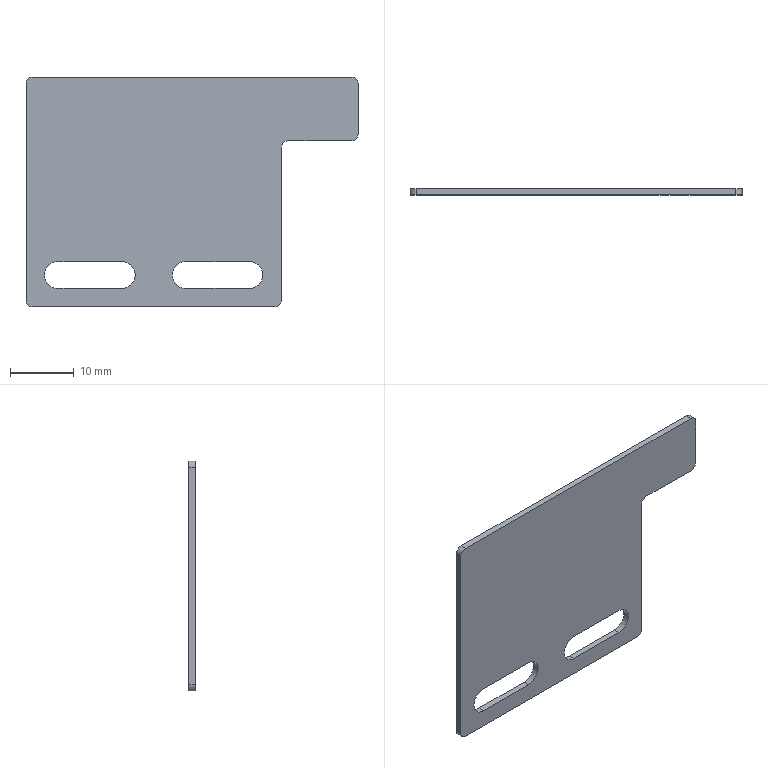Part | NX | features BREP 1 | 1 solid | 24 faces | box 52 x 1 x 36 mm | volume 1447 mm3 | cylinder 12 | plane 12 | commonest cylinder face diameters 2 x6 4.2 x6
STEP:
#1=CARTESIAN_POINT('',(20.,0.,1.));
#2=VERTEX_POINT('',#1);
#3=CARTESIAN_POINT('',(19.,0.,0.));
#4=VERTEX_POINT('',#3);
#5=CARTESIAN_POINT('',(19.,0.,1.));
#6=DIRECTION('',(0.,1.,0.));
#7=DIRECTION('',(-1.,0.,0.));
#8=AXIS2_PLACEMENT_3D('',#5,#6,#7);
#9=CIRCLE('',#8,1.);
#10=EDGE_CURVE('',#2,#4,#9,.T.);
#11=ORIENTED_EDGE('',*,*,#10,.F.);
#12=CARTESIAN_POINT('',(20.,-1.,1.));
#13=VERTEX_POINT('',#12);
#14=CARTESIAN_POINT('',(20.,0.,1.));
#15=DIRECTION('',(0.,1.,0.));
#16=VECTOR('',#15,1000.);
#17=LINE('',#14,#16);
#18=EDGE_CURVE('',#13,#2,#17,.T.);
#19=ORIENTED_EDGE('',*,*,#18,.F.);
#20=CARTESIAN_POINT('',(19.,-1.,0.));
#21=VERTEX_POINT('',#20);
#22=CARTESIAN_POINT('',(19.,-1.,1.));
#23=DIRECTION('',(0.,-1.,0.));
#24=DIRECTION('',(-1.,0.,0.));
#25=AXIS2_PLACEMENT_3D('',#22,#23,#24);
#26=CIRCLE('',#25,1.);
#27=EDGE_CURVE('',#21,#13,#26,.T.);
#28=ORIENTED_EDGE('',*,*,#27,.F.);
#29=CARTESIAN_POINT('',(19.,0.,0.));
#30=DIRECTION('',(0.,-1.,0.));
#31=VECTOR('',#30,1000.);
#32=LINE('',#29,#31);
#33=EDGE_CURVE('',#4,#21,#32,.T.);
#34=ORIENTED_EDGE('',*,*,#33,.F.);
#35=EDGE_LOOP('',(#11,#19,#28,#34));
#36=FACE_BOUND('',#35,.T.);
#37=CARTESIAN_POINT('',(19.,0.,1.));
#38=DIRECTION('',(0.,-1.,0.));
#39=DIRECTION('',(0.,0.,-1.));
#40=AXIS2_PLACEMENT_3D('',#37,#38,#39);
#41=CYLINDRICAL_SURFACE('',#40,1.);
#42=ADVANCED_FACE('',(#36),#41,.T.);
#43=CARTESIAN_POINT('',(-20.,-1.,1.));
#44=VERTEX_POINT('',#43);
#45=CARTESIAN_POINT('',(-19.,-1.,0.));
#46=VERTEX_POINT('',#45);
#47=CARTESIAN_POINT('',(-19.,-1.,1.));
#48=DIRECTION('',(0.,-1.,0.));
#49=DIRECTION('',(-1.,0.,0.));
#50=AXIS2_PLACEMENT_3D('',#47,#48,#49);
#51=CIRCLE('',#50,1.);
#52=EDGE_CURVE('',#44,#46,#51,.T.);
#53=ORIENTED_EDGE('',*,*,#52,.F.);
#54=CARTESIAN_POINT('',(-20.,0.,1.));
#55=VERTEX_POINT('',#54);
#56=CARTESIAN_POINT('',(-20.,-1.,1.));
#57=DIRECTION('',(0.,-1.,0.));
#58=VECTOR('',#57,1000.);
#59=LINE('',#56,#58);
#60=EDGE_CURVE('',#55,#44,#59,.T.);
#61=ORIENTED_EDGE('',*,*,#60,.F.);
#62=CARTESIAN_POINT('',(-19.,0.,0.));
#63=VERTEX_POINT('',#62);
#64=CARTESIAN_POINT('',(-19.,0.,1.));
#65=DIRECTION('',(0.,1.,0.));
#66=DIRECTION('',(-1.,0.,0.));
#67=AXIS2_PLACEMENT_3D('',#64,#65,#66);
#68=CIRCLE('',#67,1.);
#69=EDGE_CURVE('',#63,#55,#68,.T.);
#70=ORIENTED_EDGE('',*,*,#69,.F.);
#71=CARTESIAN_POINT('',(-19.,0.,0.));
#72=DIRECTION('',(0.,1.,0.));
#73=VECTOR('',#72,1000.);
#74=LINE('',#71,#73);
#75=EDGE_CURVE('',#46,#63,#74,.T.);
#76=ORIENTED_EDGE('',*,*,#75,.F.);
#77=EDGE_LOOP('',(#53,#61,#70,#76));
#78=FACE_BOUND('',#77,.T.);
#79=CARTESIAN_POINT('',(-19.,0.,1.));
#80=DIRECTION('',(0.,1.,0.));
#81=DIRECTION('',(0.,0.,1.));
#82=AXIS2_PLACEMENT_3D('',#79,#80,#81);
#83=CYLINDRICAL_SURFACE('',#82,1.);
#84=ADVANCED_FACE('',(#78),#83,.T.);
#85=CARTESIAN_POINT('',(20.,-1.,25.));
#86=VERTEX_POINT('',#85);
#87=CARTESIAN_POINT('',(21.,-1.,26.));
#88=VERTEX_POINT('',#87);
#89=CARTESIAN_POINT('',(21.,-1.,25.));
#90=DIRECTION('',(0.,1.,0.));
#91=DIRECTION('',(-1.,0.,0.));
#92=AXIS2_PLACEMENT_3D('',#89,#90,#91);
#93=CIRCLE('',#92,1.);
#94=EDGE_CURVE('',#86,#88,#93,.T.);
#95=ORIENTED_EDGE('',*,*,#94,.F.);
#96=CARTESIAN_POINT('',(20.,0.,25.));
#97=VERTEX_POINT('',#96);
#98=CARTESIAN_POINT('',(20.,-1.,25.));
#99=DIRECTION('',(0.,-1.,0.));
#100=VECTOR('',#99,1000.);
#101=LINE('',#98,#100);
#102=EDGE_CURVE('',#97,#86,#101,.T.);
#103=ORIENTED_EDGE('',*,*,#102,.F.);
#104=CARTESIAN_POINT('',(21.,0.,26.));
#105=VERTEX_POINT('',#104);
#106=CARTESIAN_POINT('',(21.,0.,25.));
#107=DIRECTION('',(0.,-1.,0.));
#108=DIRECTION('',(-1.,0.,0.));
#109=AXIS2_PLACEMENT_3D('',#106,#107,#108);
#110=CIRCLE('',#109,1.);
#111=EDGE_CURVE('',#105,#97,#110,.T.);
#112=ORIENTED_EDGE('',*,*,#111,.F.);
#113=CARTESIAN_POINT('',(21.,0.,26.));
#114=DIRECTION('',(0.,1.,0.));
#115=VECTOR('',#114,1000.);
#116=LINE('',#113,#115);
#117=EDGE_CURVE('',#88,#105,#116,.T.);
#118=ORIENTED_EDGE('',*,*,#117,.F.);
#119=EDGE_LOOP('',(#95,#103,#112,#118));
#120=FACE_BOUND('',#119,.T.);
#121=CARTESIAN_POINT('',(21.,-1.,25.));
#122=DIRECTION('',(0.,-1.,0.));
#123=DIRECTION('',(0.,0.,-1.));
#124=AXIS2_PLACEMENT_3D('',#121,#122,#123);
#125=CYLINDRICAL_SURFACE('',#124,1.);
#126=ADVANCED_FACE('',(#120),#125,.F.);
#127=CARTESIAN_POINT('',(31.,-1.,26.));
#128=VERTEX_POINT('',#127);
#129=CARTESIAN_POINT('',(32.,-1.,27.));
#130=VERTEX_POINT('',#129);
#131=CARTESIAN_POINT('',(31.,-1.,27.));
#132=DIRECTION('',(0.,-1.,0.));
#133=DIRECTION('',(-1.,0.,0.));
#134=AXIS2_PLACEMENT_3D('',#131,#132,#133);
#135=CIRCLE('',#134,1.);
#136=EDGE_CURVE('',#128,#130,#135,.T.);
#137=ORIENTED_EDGE('',*,*,#136,.F.);
#138=CARTESIAN_POINT('',(31.,0.,26.));
#139=VERTEX_POINT('',#138);
#140=CARTESIAN_POINT('',(31.,-1.,26.));
#141=DIRECTION('',(0.,-1.,0.));
#142=VECTOR('',#141,1000.);
#143=LINE('',#140,#142);
#144=EDGE_CURVE('',#139,#128,#143,.T.);
#145=ORIENTED_EDGE('',*,*,#144,.F.);
#146=CARTESIAN_POINT('',(32.,0.,27.));
#147=VERTEX_POINT('',#146);
#148=CARTESIAN_POINT('',(31.,0.,27.));
#149=DIRECTION('',(0.,1.,0.));
#150=DIRECTION('',(-1.,0.,0.));
#151=AXIS2_PLACEMENT_3D('',#148,#149,#150);
#152=CIRCLE('',#151,1.);
#153=EDGE_CURVE('',#147,#139,#152,.T.);
#154=ORIENTED_EDGE('',*,*,#153,.F.);
#155=CARTESIAN_POINT('',(32.,-1.,27.));
#156=DIRECTION('',(0.,1.,0.));
#157=VECTOR('',#156,1000.);
#158=LINE('',#155,#157);
#159=EDGE_CURVE('',#130,#147,#158,.T.);
#160=ORIENTED_EDGE('',*,*,#159,.F.);
#161=EDGE_LOOP('',(#137,#145,#154,#160));
#162=FACE_BOUND('',#161,.T.);
#163=CARTESIAN_POINT('',(31.,-1.,27.));
#164=DIRECTION('',(0.,1.,0.));
#165=DIRECTION('',(-1.,0.,0.));
#166=AXIS2_PLACEMENT_3D('',#163,#164,#165);
#167=CYLINDRICAL_SURFACE('',#166,1.);
#168=ADVANCED_FACE('',(#162),#167,.T.);
#169=CARTESIAN_POINT('',(32.,-1.,35.));
#170=VERTEX_POINT('',#169);
#171=CARTESIAN_POINT('',(31.,-1.,36.));
#172=VERTEX_POINT('',#171);
#173=CARTESIAN_POINT('',(31.,-1.,35.));
#174=DIRECTION('',(0.,-1.,0.));
#175=DIRECTION('',(-1.,0.,0.));
#176=AXIS2_PLACEMENT_3D('',#173,#174,#175);
#177=CIRCLE('',#176,1.);
#178=EDGE_CURVE('',#170,#172,#177,.T.);
#179=ORIENTED_EDGE('',*,*,#178,.F.);
#180=CARTESIAN_POINT('',(32.,0.,35.));
#181=VERTEX_POINT('',#180);
#182=CARTESIAN_POINT('',(32.,-1.,35.));
#183=DIRECTION('',(0.,-1.,0.));
#184=VECTOR('',#183,1000.);
#185=LINE('',#182,#184);
#186=EDGE_CURVE('',#181,#170,#185,.T.);
#187=ORIENTED_EDGE('',*,*,#186,.F.);
#188=CARTESIAN_POINT('',(31.,0.,36.));
#189=VERTEX_POINT('',#188);
#190=CARTESIAN_POINT('',(31.,0.,35.));
#191=DIRECTION('',(0.,1.,0.));
#192=DIRECTION('',(-1.,0.,0.));
#193=AXIS2_PLACEMENT_3D('',#190,#191,#192);
#194=CIRCLE('',#193,1.);
#195=EDGE_CURVE('',#189,#181,#194,.T.);
#196=ORIENTED_EDGE('',*,*,#195,.F.);
#197=CARTESIAN_POINT('',(31.,0.,36.));
#198=DIRECTION('',(0.,1.,0.));
#199=VECTOR('',#198,1000.);
#200=LINE('',#197,#199);
#201=EDGE_CURVE('',#172,#189,#200,.T.);
#202=ORIENTED_EDGE('',*,*,#201,.F.);
#203=EDGE_LOOP('',(#179,#187,#196,#202));
#204=FACE_BOUND('',#203,.T.);
#205=CARTESIAN_POINT('',(31.,0.,35.));
#206=DIRECTION('',(0.,-1.,0.));
#207=DIRECTION('',(1.,0.,0.));
#208=AXIS2_PLACEMENT_3D('',#205,#206,#207);
#209=CYLINDRICAL_SURFACE('',#208,1.);
#210=ADVANCED_FACE('',(#204),#209,.T.);
#211=CARTESIAN_POINT('',(-19.,-1.,36.));
#212=VERTEX_POINT('',#211);
#213=CARTESIAN_POINT('',(-20.,-1.,35.));
#214=VERTEX_POINT('',#213);
#215=CARTESIAN_POINT('',(-19.,-1.,35.));
#216=DIRECTION('',(0.,-1.,0.));
#217=DIRECTION('',(-1.,0.,0.));
#218=AXIS2_PLACEMENT_3D('',#215,#216,#217);
#219=CIRCLE('',#218,1.);
#220=EDGE_CURVE('',#212,#214,#219,.T.);
#221=ORIENTED_EDGE('',*,*,#220,.F.);
#222=CARTESIAN_POINT('',(-19.,0.,36.));
#223=VERTEX_POINT('',#222);
#224=CARTESIAN_POINT('',(-19.,-1.,36.));
#225=DIRECTION('',(0.,-1.,0.));
#226=VECTOR('',#225,1000.);
#227=LINE('',#224,#226);
#228=EDGE_CURVE('',#223,#212,#227,.T.);
#229=ORIENTED_EDGE('',*,*,#228,.F.);
#230=CARTESIAN_POINT('',(-20.,0.,35.));
#231=VERTEX_POINT('',#230);
#232=CARTESIAN_POINT('',(-19.,0.,35.));
#233=DIRECTION('',(0.,1.,0.));
#234=DIRECTION('',(-1.,0.,0.));
#235=AXIS2_PLACEMENT_3D('',#232,#233,#234);
#236=CIRCLE('',#235,1.);
#237=EDGE_CURVE('',#231,#223,#236,.T.);
#238=ORIENTED_EDGE('',*,*,#237,.F.);
#239=CARTESIAN_POINT('',(-20.,0.,35.));
#240=DIRECTION('',(0.,1.,0.));
#241=VECTOR('',#240,1000.);
#242=LINE('',#239,#241);
#243=EDGE_CURVE('',#214,#231,#242,.T.);
#244=ORIENTED_EDGE('',*,*,#243,.F.);
#245=EDGE_LOOP('',(#221,#229,#238,#244));
#246=FACE_BOUND('',#245,.T.);
#247=CARTESIAN_POINT('',(-19.,-1.,35.));
#248=DIRECTION('',(0.,-1.,0.));
#249=DIRECTION('',(0.,0.,-1.));
#250=AXIS2_PLACEMENT_3D('',#247,#248,#249);
#251=CYLINDRICAL_SURFACE('',#250,1.);
#252=ADVANCED_FACE('',(#246),#251,.T.);
#253=CARTESIAN_POINT('',(32.,0.,36.));
#254=DIRECTION('',(0.,0.,-1.));
#255=VECTOR('',#254,1000.);
#256=LINE('',#253,#255);
#257=EDGE_CURVE('',#181,#147,#256,.T.);
#258=ORIENTED_EDGE('',*,*,#257,.F.);
#259=ORIENTED_EDGE('',*,*,#186,.T.);
#260=CARTESIAN_POINT('',(32.,-1.,36.));
#261=DIRECTION('',(0.,0.,-1.));
#262=VECTOR('',#261,1000.);
#263=LINE('',#260,#262);
#264=EDGE_CURVE('',#170,#130,#263,.T.);
#265=ORIENTED_EDGE('',*,*,#264,.T.);
#266=ORIENTED_EDGE('',*,*,#159,.T.);
#267=EDGE_LOOP('',(#258,#259,#265,#266));
#268=FACE_BOUND('',#267,.T.);
#269=CARTESIAN_POINT('',(32.,-1.,36.));
#270=DIRECTION('',(1.,0.,0.));
#271=DIRECTION('',(0.,1.,0.));
#272=AXIS2_PLACEMENT_3D('',#269,#270,#271);
#273=PLANE('',#272);
#274=ADVANCED_FACE('',(#268),#273,.T.);
#275=CARTESIAN_POINT('',(32.,0.,26.));
#276=DIRECTION('',(-1.,0.,0.));
#277=VECTOR('',#276,1000.);
#278=LINE('',#275,#277);
#279=EDGE_CURVE('',#139,#105,#278,.T.);
#280=ORIENTED_EDGE('',*,*,#279,.F.);
#281=ORIENTED_EDGE('',*,*,#144,.T.);
#282=CARTESIAN_POINT('',(32.,-1.,26.));
#283=DIRECTION('',(-1.,0.,0.));
#284=VECTOR('',#283,1000.);
#285=LINE('',#282,#284);
#286=EDGE_CURVE('',#128,#88,#285,.T.);
#287=ORIENTED_EDGE('',*,*,#286,.T.);
#288=ORIENTED_EDGE('',*,*,#117,.T.);
#289=EDGE_LOOP('',(#280,#281,#287,#288));
#290=FACE_BOUND('',#289,.T.);
#291=CARTESIAN_POINT('',(32.,-1.,26.));
#292=DIRECTION('',(0.,0.,-1.));
#293=DIRECTION('',(-1.,0.,0.));
#294=AXIS2_PLACEMENT_3D('',#291,#292,#293);
#295=PLANE('',#294);
#296=ADVANCED_FACE('',(#290),#295,.T.);
#297=CARTESIAN_POINT('',(5.,-1.,7.1));
#298=VERTEX_POINT('',#297);
#299=CARTESIAN_POINT('',(5.,0.,7.1));
#300=VERTEX_POINT('',#299);
#301=CARTESIAN_POINT('',(5.,-10.,7.1));
#302=DIRECTION('',(0.,1.,0.));
#303=VECTOR('',#302,1000.);
#304=LINE('',#301,#303);
#305=EDGE_CURVE('',#298,#300,#304,.T.);
#306=ORIENTED_EDGE('',*,*,#305,.T.);
#307=CARTESIAN_POINT('',(15.,0.,7.1));
#308=VERTEX_POINT('',#307);
#309=CARTESIAN_POINT('',(5.,0.,7.1));
#310=DIRECTION('',(1.,0.,0.));
#311=VECTOR('',#310,1000.);
#312=LINE('',#309,#311);
#313=EDGE_CURVE('',#300,#308,#312,.T.);
#314=ORIENTED_EDGE('',*,*,#313,.T.);
#315=CARTESIAN_POINT('',(15.,-1.,7.1));
#316=VERTEX_POINT('',#315);
#317=CARTESIAN_POINT('',(15.,-10.,7.1));
#318=DIRECTION('',(0.,1.,0.));
#319=VECTOR('',#318,1000.);
#320=LINE('',#317,#319);
#321=EDGE_CURVE('',#316,#308,#320,.T.);
#322=ORIENTED_EDGE('',*,*,#321,.F.);
#323=CARTESIAN_POINT('',(-20.,-1.,7.1));
#324=DIRECTION('',(1.,0.,0.));
#325=VECTOR('',#324,1000.);
#326=LINE('',#323,#325);
#327=EDGE_CURVE('',#298,#316,#326,.T.);
#328=ORIENTED_EDGE('',*,*,#327,.F.);
#329=EDGE_LOOP('',(#306,#314,#322,#328));
#330=FACE_BOUND('',#329,.T.);
#331=CARTESIAN_POINT('',(5.,-10.,7.1));
#332=DIRECTION('',(0.,0.,1.));
#333=DIRECTION('',(1.,0.,0.));
#334=AXIS2_PLACEMENT_3D('',#331,#332,#333);
#335=PLANE('',#334);
#336=ADVANCED_FACE('',(#330),#335,.F.);
#337=ORIENTED_EDGE('',*,*,#321,.T.);
#338=CARTESIAN_POINT('',(15.,0.,2.9));
#339=VERTEX_POINT('',#338);
#340=CARTESIAN_POINT('',(15.,0.,5.));
#341=DIRECTION('',(0.,1.,0.));
#342=DIRECTION('',(-1.,0.,0.));
#343=AXIS2_PLACEMENT_3D('',#340,#341,#342);
#344=CIRCLE('',#343,2.1);
#345=EDGE_CURVE('',#308,#339,#344,.T.);
#346=ORIENTED_EDGE('',*,*,#345,.T.);
#347=CARTESIAN_POINT('',(15.,-1.,2.9));
#348=VERTEX_POINT('',#347);
#349=CARTESIAN_POINT('',(15.,-10.,2.9));
#350=DIRECTION('',(0.,1.,0.));
#351=VECTOR('',#350,1000.);
#352=LINE('',#349,#351);
#353=EDGE_CURVE('',#348,#339,#352,.T.);
#354=ORIENTED_EDGE('',*,*,#353,.F.);
#355=CARTESIAN_POINT('',(15.,-1.,5.));
#356=DIRECTION('',(0.,1.,0.));
#357=DIRECTION('',(-1.,0.,0.));
#358=AXIS2_PLACEMENT_3D('',#355,#356,#357);
#359=CIRCLE('',#358,2.1);
#360=EDGE_CURVE('',#316,#348,#359,.T.);
#361=ORIENTED_EDGE('',*,*,#360,.F.);
#362=EDGE_LOOP('',(#337,#346,#354,#361));
#363=FACE_BOUND('',#362,.T.);
#364=CARTESIAN_POINT('',(15.,-10.,5.));
#365=DIRECTION('',(0.,1.,0.));
#366=DIRECTION('',(-1.,0.,0.));
#367=AXIS2_PLACEMENT_3D('',#364,#365,#366);
#368=CYLINDRICAL_SURFACE('',#367,2.1);
#369=ADVANCED_FACE('',(#363),#368,.F.);
#370=ORIENTED_EDGE('',*,*,#353,.T.);
#371=CARTESIAN_POINT('',(5.,0.,2.9));
#372=VERTEX_POINT('',#371);
#373=CARTESIAN_POINT('',(5.,0.,2.9));
#374=DIRECTION('',(-1.,0.,0.));
#375=VECTOR('',#374,1000.);
#376=LINE('',#373,#375);
#377=EDGE_CURVE('',#339,#372,#376,.T.);
#378=ORIENTED_EDGE('',*,*,#377,.T.);
#379=CARTESIAN_POINT('',(5.,-1.,2.9));
#380=VERTEX_POINT('',#379);
#381=CARTESIAN_POINT('',(5.,-10.,2.9));
#382=DIRECTION('',(0.,1.,0.));
#383=VECTOR('',#382,1000.);
#384=LINE('',#381,#383);
#385=EDGE_CURVE('',#380,#372,#384,.T.);
#386=ORIENTED_EDGE('',*,*,#385,.F.);
#387=CARTESIAN_POINT('',(-20.,-1.,2.9));
#388=DIRECTION('',(-1.,0.,0.));
#389=VECTOR('',#388,1000.);
#390=LINE('',#387,#389);
#391=EDGE_CURVE('',#348,#380,#390,.T.);
#392=ORIENTED_EDGE('',*,*,#391,.F.);
#393=EDGE_LOOP('',(#370,#378,#386,#392));
#394=FACE_BOUND('',#393,.T.);
#395=CARTESIAN_POINT('',(5.,-10.,2.9));
#396=DIRECTION('',(0.,0.,-1.));
#397=DIRECTION('',(-1.,0.,0.));
#398=AXIS2_PLACEMENT_3D('',#395,#396,#397);
#399=PLANE('',#398);
#400=ADVANCED_FACE('',(#394),#399,.F.);
#401=CARTESIAN_POINT('',(2.9,-1.,5.));
#402=VERTEX_POINT('',#401);
#403=CARTESIAN_POINT('',(2.9,0.,5.));
#404=VERTEX_POINT('',#403);
#405=CARTESIAN_POINT('',(2.9,-10.,5.));
#406=DIRECTION('',(0.,1.,0.));
#407=VECTOR('',#406,1000.);
#408=LINE('',#405,#407);
#409=EDGE_CURVE('',#402,#404,#408,.T.);
#410=ORIENTED_EDGE('',*,*,#409,.F.);
#411=CARTESIAN_POINT('',(5.,-1.,5.));
#412=DIRECTION('',(0.,1.,0.));
#413=DIRECTION('',(-1.,0.,0.));
#414=AXIS2_PLACEMENT_3D('',#411,#412,#413);
#415=CIRCLE('',#414,2.1);
#416=EDGE_CURVE('',#380,#402,#415,.T.);
#417=ORIENTED_EDGE('',*,*,#416,.F.);
#418=ORIENTED_EDGE('',*,*,#385,.T.);
#419=CARTESIAN_POINT('',(5.,0.,5.));
#420=DIRECTION('',(0.,1.,0.));
#421=DIRECTION('',(-1.,0.,0.));
#422=AXIS2_PLACEMENT_3D('',#419,#420,#421);
#423=CIRCLE('',#422,2.1);
#424=EDGE_CURVE('',#372,#404,#423,.T.);
#425=ORIENTED_EDGE('',*,*,#424,.T.);
#426=EDGE_LOOP('',(#410,#417,#418,#425));
#427=FACE_BOUND('',#426,.T.);
#428=CARTESIAN_POINT('',(5.,-10.,5.));
#429=DIRECTION('',(0.,1.,0.));
#430=DIRECTION('',(-1.,0.,0.));
#431=AXIS2_PLACEMENT_3D('',#428,#429,#430);
#432=CYLINDRICAL_SURFACE('',#431,2.1);
#433=ADVANCED_FACE('',(#427),#432,.F.);
#434=CARTESIAN_POINT('',(-15.,-1.,7.1));
#435=VERTEX_POINT('',#434);
#436=CARTESIAN_POINT('',(-15.,0.,7.1));
#437=VERTEX_POINT('',#436);
#438=CARTESIAN_POINT('',(-15.,-10.,7.1));
#439=DIRECTION('',(0.,1.,0.));
#440=VECTOR('',#439,1000.);
#441=LINE('',#438,#440);
#442=EDGE_CURVE('',#435,#437,#441,.T.);
#443=ORIENTED_EDGE('',*,*,#442,.T.);
#444=CARTESIAN_POINT('',(-5.,0.,7.1));
#445=VERTEX_POINT('',#444);
#446=CARTESIAN_POINT('',(-15.,0.,7.1));
#447=DIRECTION('',(1.,0.,0.));
#448=VECTOR('',#447,1000.);
#449=LINE('',#446,#448);
#450=EDGE_CURVE('',#437,#445,#449,.T.);
#451=ORIENTED_EDGE('',*,*,#450,.T.);
#452=CARTESIAN_POINT('',(-5.,-1.,7.1));
#453=VERTEX_POINT('',#452);
#454=CARTESIAN_POINT('',(-5.,-10.,7.1));
#455=DIRECTION('',(0.,1.,0.));
#456=VECTOR('',#455,1000.);
#457=LINE('',#454,#456);
#458=EDGE_CURVE('',#453,#445,#457,.T.);
#459=ORIENTED_EDGE('',*,*,#458,.F.);
#460=CARTESIAN_POINT('',(-20.,-1.,7.1));
#461=DIRECTION('',(1.,0.,0.));
#462=VECTOR('',#461,1000.);
#463=LINE('',#460,#462);
#464=EDGE_CURVE('',#435,#453,#463,.T.);
#465=ORIENTED_EDGE('',*,*,#464,.F.);
#466=EDGE_LOOP('',(#443,#451,#459,#465));
#467=FACE_BOUND('',#466,.T.);
#468=CARTESIAN_POINT('',(-15.,-10.,7.1));
#469=DIRECTION('',(0.,0.,1.));
#470=DIRECTION('',(1.,0.,0.));
#471=AXIS2_PLACEMENT_3D('',#468,#469,#470);
#472=PLANE('',#471);
#473=ADVANCED_FACE('',(#467),#472,.F.);
#474=ORIENTED_EDGE('',*,*,#458,.T.);
#475=CARTESIAN_POINT('',(-5.,0.,2.9));
#476=VERTEX_POINT('',#475);
#477=CARTESIAN_POINT('',(-5.,0.,5.));
#478=DIRECTION('',(0.,1.,0.));
#479=DIRECTION('',(-1.,0.,0.));
#480=AXIS2_PLACEMENT_3D('',#477,#478,#479);
#481=CIRCLE('',#480,2.1);
#482=EDGE_CURVE('',#445,#476,#481,.T.);
#483=ORIENTED_EDGE('',*,*,#482,.T.);
#484=CARTESIAN_POINT('',(-5.,-1.,2.9));
#485=VERTEX_POINT('',#484);
#486=CARTESIAN_POINT('',(-5.,-10.,2.9));
#487=DIRECTION('',(0.,1.,0.));
#488=VECTOR('',#487,1000.);
#489=LINE('',#486,#488);
#490=EDGE_CURVE('',#485,#476,#489,.T.);
#491=ORIENTED_EDGE('',*,*,#490,.F.);
#492=CARTESIAN_POINT('',(-5.,-1.,5.));
#493=DIRECTION('',(0.,1.,0.));
#494=DIRECTION('',(-1.,0.,0.));
#495=AXIS2_PLACEMENT_3D('',#492,#493,#494);
#496=CIRCLE('',#495,2.1);
#497=EDGE_CURVE('',#453,#485,#496,.T.);
#498=ORIENTED_EDGE('',*,*,#497,.F.);
#499=EDGE_LOOP('',(#474,#483,#491,#498));
#500=FACE_BOUND('',#499,.T.);
#501=CARTESIAN_POINT('',(-5.,-10.,5.));
#502=DIRECTION('',(0.,1.,0.));
#503=DIRECTION('',(-1.,0.,0.));
#504=AXIS2_PLACEMENT_3D('',#501,#502,#503);
#505=CYLINDRICAL_SURFACE('',#504,2.1);
#506=ADVANCED_FACE('',(#500),#505,.F.);
#507=ORIENTED_EDGE('',*,*,#490,.T.);
#508=CARTESIAN_POINT('',(-15.,0.,2.9));
#509=VERTEX_POINT('',#508);
#510=CARTESIAN_POINT('',(-15.,0.,2.9));
#511=DIRECTION('',(-1.,0.,0.));
#512=VECTOR('',#511,1000.);
#513=LINE('',#510,#512);
#514=EDGE_CURVE('',#476,#509,#513,.T.);
#515=ORIENTED_EDGE('',*,*,#514,.T.);
#516=CARTESIAN_POINT('',(-15.,-1.,2.9));
#517=VERTEX_POINT('',#516);
#518=CARTESIAN_POINT('',(-15.,-10.,2.9));
#519=DIRECTION('',(0.,1.,0.));
#520=VECTOR('',#519,1000.);
#521=LINE('',#518,#520);
#522=EDGE_CURVE('',#517,#509,#521,.T.);
#523=ORIENTED_EDGE('',*,*,#522,.F.);
#524=CARTESIAN_POINT('',(-20.,-1.,2.9));
#525=DIRECTION('',(-1.,0.,0.));
#526=VECTOR('',#525,1000.);
#527=LINE('',#524,#526);
#528=EDGE_CURVE('',#485,#517,#527,.T.);
#529=ORIENTED_EDGE('',*,*,#528,.F.);
#530=EDGE_LOOP('',(#507,#515,#523,#529));
#531=FACE_BOUND('',#530,.T.);
#532=CARTESIAN_POINT('',(-15.,-10.,2.9));
#533=DIRECTION('',(0.,0.,-1.));
#534=DIRECTION('',(-1.,0.,0.));
#535=AXIS2_PLACEMENT_3D('',#532,#533,#534);
#536=PLANE('',#535);
#537=ADVANCED_FACE('',(#531),#536,.F.);
#538=CARTESIAN_POINT('',(-17.1,-1.,5.));
#539=VERTEX_POINT('',#538);
#540=CARTESIAN_POINT('',(-17.1,0.,5.));
#541=VERTEX_POINT('',#540);
#542=CARTESIAN_POINT('',(-17.1,-10.,5.));
#543=DIRECTION('',(0.,1.,0.));
#544=VECTOR('',#543,1000.);
#545=LINE('',#542,#544);
#546=EDGE_CURVE('',#539,#541,#545,.T.);
#547=ORIENTED_EDGE('',*,*,#546,.F.);
#548=CARTESIAN_POINT('',(-15.,-1.,5.));
#549=DIRECTION('',(0.,1.,0.));
#550=DIRECTION('',(-1.,0.,0.));
#551=AXIS2_PLACEMENT_3D('',#548,#549,#550);
#552=CIRCLE('',#551,2.1);
#553=EDGE_CURVE('',#517,#539,#552,.T.);
#554=ORIENTED_EDGE('',*,*,#553,.F.);
#555=ORIENTED_EDGE('',*,*,#522,.T.);
#556=CARTESIAN_POINT('',(-15.,0.,5.));
#557=DIRECTION('',(0.,1.,0.));
#558=DIRECTION('',(-1.,0.,0.));
#559=AXIS2_PLACEMENT_3D('',#556,#557,#558);
#560=CIRCLE('',#559,2.1);
#561=EDGE_CURVE('',#509,#541,#560,.T.);
#562=ORIENTED_EDGE('',*,*,#561,.T.);
#563=EDGE_LOOP('',(#547,#554,#555,#562));
#564=FACE_BOUND('',#563,.T.);
#565=CARTESIAN_POINT('',(-15.,-10.,5.));
#566=DIRECTION('',(0.,1.,0.));
#567=DIRECTION('',(-1.,0.,0.));
#568=AXIS2_PLACEMENT_3D('',#565,#566,#567);
#569=CYLINDRICAL_SURFACE('',#568,2.1);
#570=ADVANCED_FACE('',(#564),#569,.F.);
#571=CARTESIAN_POINT('',(-20.,-1.,0.));
#572=DIRECTION('',(1.,0.,0.));
#573=VECTOR('',#572,1000.);
#574=LINE('',#571,#573);
#575=EDGE_CURVE('',#46,#21,#574,.T.);
#576=ORIENTED_EDGE('',*,*,#575,.F.);
#577=ORIENTED_EDGE('',*,*,#75,.T.);
#578=CARTESIAN_POINT('',(-20.,0.,0.));
#579=DIRECTION('',(1.,0.,0.));
#580=VECTOR('',#579,1000.);
#581=LINE('',#578,#580);
#582=EDGE_CURVE('',#63,#4,#581,.T.);
#583=ORIENTED_EDGE('',*,*,#582,.T.);
#584=ORIENTED_EDGE('',*,*,#33,.T.);
#585=EDGE_LOOP('',(#576,#577,#583,#584));
#586=FACE_BOUND('',#585,.T.);
#587=CARTESIAN_POINT('',(0.,0.,0.));
#588=DIRECTION('',(0.,0.,-1.));
#589=DIRECTION('',(-1.,0.,0.));
#590=AXIS2_PLACEMENT_3D('',#587,#588,#589);
#591=PLANE('',#590);
#592=ADVANCED_FACE('',(#586),#591,.T.);
#593=CARTESIAN_POINT('',(-20.,0.,36.));
#594=DIRECTION('',(1.,0.,0.));
#595=VECTOR('',#594,1000.);
#596=LINE('',#593,#595);
#597=EDGE_CURVE('',#223,#189,#596,.T.);
#598=ORIENTED_EDGE('',*,*,#597,.F.);
#599=ORIENTED_EDGE('',*,*,#228,.T.);
#600=CARTESIAN_POINT('',(-20.,-1.,36.));
#601=DIRECTION('',(1.,0.,0.));
#602=VECTOR('',#601,1000.);
#603=LINE('',#600,#602);
#604=EDGE_CURVE('',#212,#172,#603,.T.);
#605=ORIENTED_EDGE('',*,*,#604,.T.);
#606=ORIENTED_EDGE('',*,*,#201,.T.);
#607=EDGE_LOOP('',(#598,#599,#605,#606));
#608=FACE_BOUND('',#607,.T.);
#609=CARTESIAN_POINT('',(0.,0.,36.));
#610=DIRECTION('',(0.,0.,-1.));
#611=DIRECTION('',(-1.,0.,0.));
#612=AXIS2_PLACEMENT_3D('',#609,#610,#611);
#613=PLANE('',#612);
#614=ADVANCED_FACE('',(#608),#613,.F.);
#615=CARTESIAN_POINT('',(-20.,-1.,36.));
#616=DIRECTION('',(0.,0.,-1.));
#617=VECTOR('',#616,1000.);
#618=LINE('',#615,#617);
#619=EDGE_CURVE('',#214,#44,#618,.T.);
#620=ORIENTED_EDGE('',*,*,#619,.F.);
#621=ORIENTED_EDGE('',*,*,#243,.T.);
#622=CARTESIAN_POINT('',(-20.,0.,36.));
#623=DIRECTION('',(0.,0.,-1.));
#624=VECTOR('',#623,1000.);
#625=LINE('',#622,#624);
#626=EDGE_CURVE('',#231,#55,#625,.T.);
#627=ORIENTED_EDGE('',*,*,#626,.T.);
#628=ORIENTED_EDGE('',*,*,#60,.T.);
#629=EDGE_LOOP('',(#620,#621,#627,#628));
#630=FACE_BOUND('',#629,.T.);
#631=CARTESIAN_POINT('',(-20.,-1.,36.));
#632=DIRECTION('',(-1.,0.,0.));
#633=DIRECTION('',(0.,0.,1.));
#634=AXIS2_PLACEMENT_3D('',#631,#632,#633);
#635=PLANE('',#634);
#636=ADVANCED_FACE('',(#630),#635,.T.);
#637=ORIENTED_EDGE('',*,*,#626,.F.);
#638=ORIENTED_EDGE('',*,*,#237,.T.);
#639=ORIENTED_EDGE('',*,*,#597,.T.);
#640=ORIENTED_EDGE('',*,*,#195,.T.);
#641=ORIENTED_EDGE('',*,*,#257,.T.);
#642=ORIENTED_EDGE('',*,*,#153,.T.);
#643=ORIENTED_EDGE('',*,*,#279,.T.);
#644=ORIENTED_EDGE('',*,*,#111,.T.);
#645=CARTESIAN_POINT('',(20.,0.,36.));
#646=DIRECTION('',(0.,0.,-1.));
#647=VECTOR('',#646,1000.);
#648=LINE('',#645,#647);
#649=EDGE_CURVE('',#97,#2,#648,.T.);
#650=ORIENTED_EDGE('',*,*,#649,.T.);
#651=ORIENTED_EDGE('',*,*,#10,.T.);
#652=ORIENTED_EDGE('',*,*,#582,.F.);
#653=ORIENTED_EDGE('',*,*,#69,.T.);
#654=EDGE_LOOP('',(#637,#638,#639,#640,#641,#642,#643,#644,#650,#651,#652,#653));
#655=FACE_BOUND('',#654,.T.);
#656=ORIENTED_EDGE('',*,*,#561,.F.);
#657=ORIENTED_EDGE('',*,*,#514,.F.);
#658=ORIENTED_EDGE('',*,*,#482,.F.);
#659=ORIENTED_EDGE('',*,*,#450,.F.);
#660=CARTESIAN_POINT('',(-15.,0.,5.));
#661=DIRECTION('',(0.,1.,0.));
#662=DIRECTION('',(-1.,0.,0.));
#663=AXIS2_PLACEMENT_3D('',#660,#661,#662);
#664=CIRCLE('',#663,2.1);
#665=EDGE_CURVE('',#541,#437,#664,.T.);
#666=ORIENTED_EDGE('',*,*,#665,.F.);
#667=EDGE_LOOP('',(#656,#657,#658,#659,#666));
#668=FACE_BOUND('',#667,.T.);
#669=ORIENTED_EDGE('',*,*,#424,.F.);
#670=ORIENTED_EDGE('',*,*,#377,.F.);
#671=ORIENTED_EDGE('',*,*,#345,.F.);
#672=ORIENTED_EDGE('',*,*,#313,.F.);
#673=CARTESIAN_POINT('',(5.,0.,5.));
#674=DIRECTION('',(0.,1.,0.));
#675=DIRECTION('',(-1.,0.,0.));
#676=AXIS2_PLACEMENT_3D('',#673,#674,#675);
#677=CIRCLE('',#676,2.1);
#678=EDGE_CURVE('',#404,#300,#677,.T.);
#679=ORIENTED_EDGE('',*,*,#678,.F.);
#680=EDGE_LOOP('',(#669,#670,#671,#672,#679));
#681=FACE_BOUND('',#680,.T.);
#682=CARTESIAN_POINT('',(-20.,0.,36.));
#683=DIRECTION('',(0.,1.,0.));
#684=DIRECTION('',(-1.,0.,0.));
#685=AXIS2_PLACEMENT_3D('',#682,#683,#684);
#686=PLANE('',#685);
#687=ADVANCED_FACE('',(#655,#668,#681),#686,.T.);
#688=ORIENTED_EDGE('',*,*,#649,.F.);
#689=ORIENTED_EDGE('',*,*,#102,.T.);
#690=CARTESIAN_POINT('',(20.,-1.,36.));
#691=DIRECTION('',(0.,0.,-1.));
#692=VECTOR('',#691,1000.);
#693=LINE('',#690,#692);
#694=EDGE_CURVE('',#86,#13,#693,.T.);
#695=ORIENTED_EDGE('',*,*,#694,.T.);
#696=ORIENTED_EDGE('',*,*,#18,.T.);
#697=EDGE_LOOP('',(#688,#689,#695,#696));
#698=FACE_BOUND('',#697,.T.);
#699=CARTESIAN_POINT('',(20.,0.,36.));
#700=DIRECTION('',(1.,0.,0.));
#701=DIRECTION('',(0.,0.,-1.));
#702=AXIS2_PLACEMENT_3D('',#699,#700,#701);
#703=PLANE('',#702);
#704=ADVANCED_FACE('',(#698),#703,.T.);
#705=ORIENTED_EDGE('',*,*,#604,.F.);
#706=ORIENTED_EDGE('',*,*,#220,.T.);
#707=ORIENTED_EDGE('',*,*,#619,.T.);
#708=ORIENTED_EDGE('',*,*,#52,.T.);
#709=ORIENTED_EDGE('',*,*,#575,.T.);
#710=ORIENTED_EDGE('',*,*,#27,.T.);
#711=ORIENTED_EDGE('',*,*,#694,.F.);
#712=ORIENTED_EDGE('',*,*,#94,.T.);
#713=ORIENTED_EDGE('',*,*,#286,.F.);
#714=ORIENTED_EDGE('',*,*,#136,.T.);
#715=ORIENTED_EDGE('',*,*,#264,.F.);
#716=ORIENTED_EDGE('',*,*,#178,.T.);
#717=EDGE_LOOP('',(#705,#706,#707,#708,#709,#710,#711,#712,#713,#714,#715,#716));
#718=FACE_BOUND('',#717,.T.);
#719=ORIENTED_EDGE('',*,*,#528,.T.);
#720=ORIENTED_EDGE('',*,*,#553,.T.);
#721=CARTESIAN_POINT('',(-15.,-1.,5.));
#722=DIRECTION('',(0.,1.,0.));
#723=DIRECTION('',(-1.,0.,0.));
#724=AXIS2_PLACEMENT_3D('',#721,#722,#723);
#725=CIRCLE('',#724,2.1);
#726=EDGE_CURVE('',#539,#435,#725,.T.);
#727=ORIENTED_EDGE('',*,*,#726,.T.);
#728=ORIENTED_EDGE('',*,*,#464,.T.);
#729=ORIENTED_EDGE('',*,*,#497,.T.);
#730=EDGE_LOOP('',(#719,#720,#727,#728,#729));
#731=FACE_BOUND('',#730,.T.);
#732=ORIENTED_EDGE('',*,*,#391,.T.);
#733=ORIENTED_EDGE('',*,*,#416,.T.);
#734=CARTESIAN_POINT('',(5.,-1.,5.));
#735=DIRECTION('',(0.,1.,0.));
#736=DIRECTION('',(-1.,0.,0.));
#737=AXIS2_PLACEMENT_3D('',#734,#735,#736);
#738=CIRCLE('',#737,2.1);
#739=EDGE_CURVE('',#402,#298,#738,.T.);
#740=ORIENTED_EDGE('',*,*,#739,.T.);
#741=ORIENTED_EDGE('',*,*,#327,.T.);
#742=ORIENTED_EDGE('',*,*,#360,.T.);
#743=EDGE_LOOP('',(#732,#733,#740,#741,#742));
#744=FACE_BOUND('',#743,.T.);
#745=CARTESIAN_POINT('',(-20.,-1.,36.));
#746=DIRECTION('',(0.,1.,0.));
#747=DIRECTION('',(-1.,0.,0.));
#748=AXIS2_PLACEMENT_3D('',#745,#746,#747);
#749=PLANE('',#748);
#750=ADVANCED_FACE('',(#718,#731,#744),#749,.F.);
#751=ORIENTED_EDGE('',*,*,#726,.F.);
#752=ORIENTED_EDGE('',*,*,#546,.T.);
#753=ORIENTED_EDGE('',*,*,#665,.T.);
#754=ORIENTED_EDGE('',*,*,#442,.F.);
#755=EDGE_LOOP('',(#751,#752,#753,#754));
#756=FACE_BOUND('',#755,.T.);
#757=CARTESIAN_POINT('',(-15.,-10.,5.));
#758=DIRECTION('',(0.,1.,0.));
#759=DIRECTION('',(-1.,0.,0.));
#760=AXIS2_PLACEMENT_3D('',#757,#758,#759);
#761=CYLINDRICAL_SURFACE('',#760,2.1);
#762=ADVANCED_FACE('',(#756),#761,.F.);
#763=ORIENTED_EDGE('',*,*,#739,.F.);
#764=ORIENTED_EDGE('',*,*,#409,.T.);
#765=ORIENTED_EDGE('',*,*,#678,.T.);
#766=ORIENTED_EDGE('',*,*,#305,.F.);
#767=EDGE_LOOP('',(#763,#764,#765,#766));
#768=FACE_BOUND('',#767,.T.);
#769=CARTESIAN_POINT('',(5.,-10.,5.));
#770=DIRECTION('',(0.,1.,0.));
#771=DIRECTION('',(-1.,0.,0.));
#772=AXIS2_PLACEMENT_3D('',#769,#770,#771);
#773=CYLINDRICAL_SURFACE('',#772,2.1);
#774=ADVANCED_FACE('',(#768),#773,.F.);
#775=CLOSED_SHELL('',(#42,#84,#126,#168,#210,#252,#274,#296,#336,#369,#400,#433,#473,#506,#537,#570,#592,#614,#636,#687,#704,#750,#762,#774));
#776=MANIFOLD_SOLID_BREP('',#775);
#777=(LENGTH_UNIT()NAMED_UNIT(*)SI_UNIT(.MILLI.,.METRE.));
#778=UNCERTAINTY_MEASURE_WITH_UNIT(LENGTH_MEASURE(0.00001),#777,'','');
#779=(NAMED_UNIT(*)PLANE_ANGLE_UNIT()SI_UNIT($,.RADIAN.));
#780=(NAMED_UNIT(*)SI_UNIT($,.STERADIAN.)SOLID_ANGLE_UNIT());
#781=(GEOMETRIC_REPRESENTATION_CONTEXT(3)GLOBAL_UNCERTAINTY_ASSIGNED_CONTEXT((#778))GLOBAL_UNIT_ASSIGNED_CONTEXT((#777,#779,#780))REPRESENTATION_CONTEXT('',''));
#782=ADVANCED_BREP_SHAPE_REPRESENTATION('',(#776),#781);